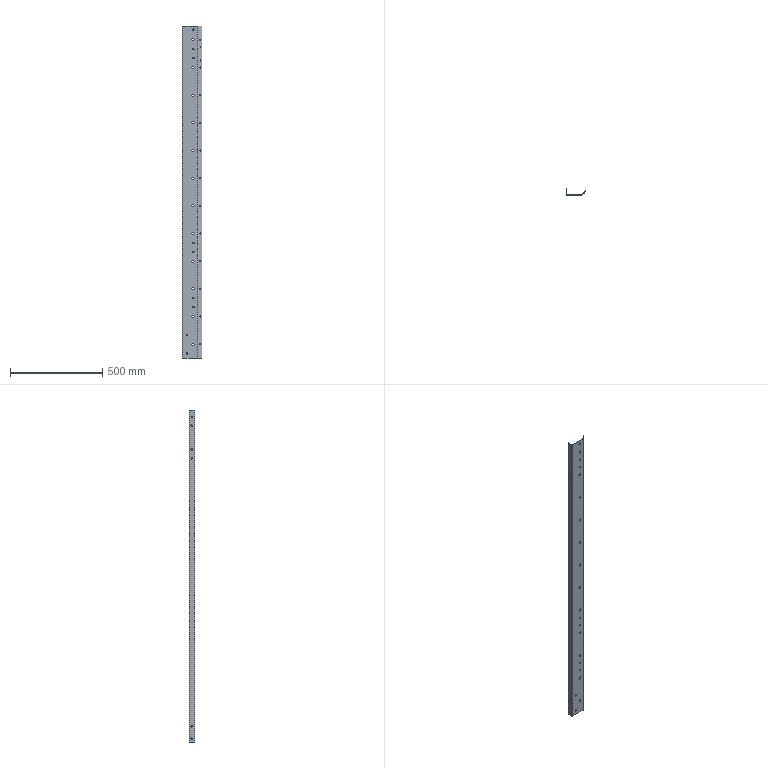Part | STEP file | Side panel wer5 N1 | 1 solid | 123 faces | box 107.981 x 30 x 1800 mm | volume 501460 mm3 | plane 90 | cylinder 33 | commonest cylinder face diameters 8.2 x22 8.5 x3 4 x2 6.5 x2 8 x2 8.3 x2